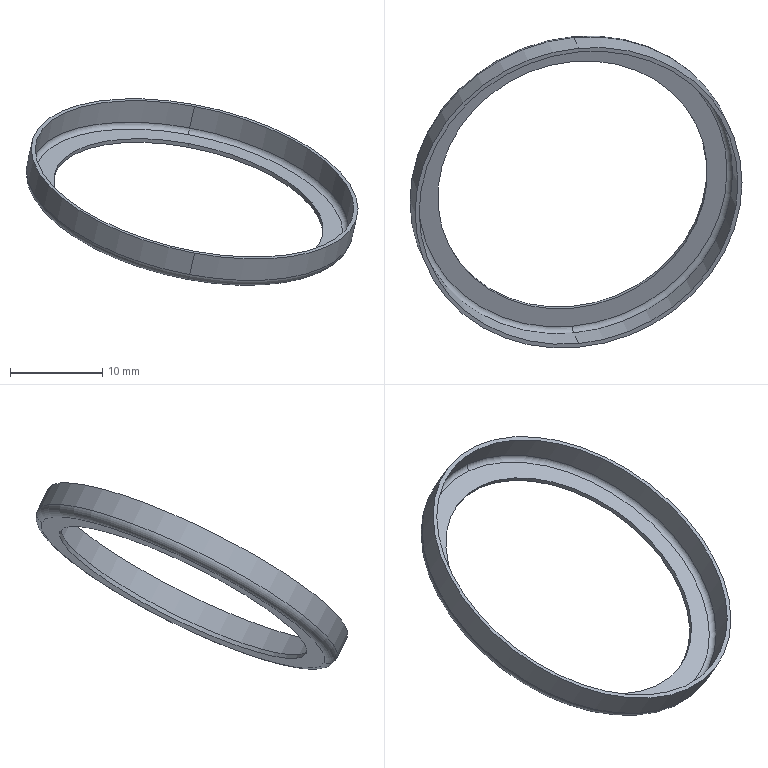Part | SolidWorks | features BaseBody 1 | 1 solid | 13 faces | box 35.944 x 33.77 x 20.198 mm | volume 291.989 mm3 | cylinder 6 | torus 4 | plane 3 | commonest cylinder face diameters 29.8 x2 35.23 x2 36.13 x2
STEP:
#1=CARTESIAN_POINT('',(1945.708,-185.265,909.185));
#2=VERTEX_POINT('',#1);
#3=CARTESIAN_POINT('',(1945.708,-211.95,895.919));
#4=VERTEX_POINT('',#3);
#5=CARTESIAN_POINT('',(1945.708,-198.607,902.552));
#6=DIRECTION('',(0.2015,-0.436,0.8771));
#7=DIRECTION('',(0.,-0.8955,-0.4451));
#8=AXIS2_PLACEMENT_3D('',#5,#6,#7);
#9=CIRCLE('',#8,14.9);
#10=EDGE_CURVE('',#2,#4,#9,.T.);
#11=ORIENTED_EDGE('',*,*,#10,.F.);
#12=CARTESIAN_POINT('',(1945.799,-185.461,909.579));
#13=VERTEX_POINT('',#12);
#14=CARTESIAN_POINT('',(1943.539,-180.572,899.743));
#15=DIRECTION('',(0.2015,-0.436,0.8771));
#16=VECTOR('',#15,1000.);
#17=LINE('',#14,#16);
#18=EDGE_CURVE('',#2,#13,#17,.T.);
#19=ORIENTED_EDGE('',*,*,#18,.T.);
#20=CARTESIAN_POINT('',(1945.799,-212.146,896.314));
#21=VERTEX_POINT('',#20);
#22=CARTESIAN_POINT('',(1945.799,-198.804,902.947));
#23=DIRECTION('',(0.2015,-0.436,0.8771));
#24=DIRECTION('',(0.,-0.8955,-0.4451));
#25=AXIS2_PLACEMENT_3D('',#22,#23,#24);
#26=CIRCLE('',#25,14.9);
#27=EDGE_CURVE('',#13,#21,#26,.T.);
#28=ORIENTED_EDGE('',*,*,#27,.T.);
#29=CARTESIAN_POINT('',(1943.539,-207.256,886.478));
#30=DIRECTION('',(0.2015,-0.436,0.8771));
#31=VECTOR('',#30,1000.);
#32=LINE('',#29,#31);
#33=EDGE_CURVE('',#4,#21,#32,.T.);
#34=ORIENTED_EDGE('',*,*,#33,.F.);
#35=EDGE_LOOP('',(#11,#19,#28,#34));
#36=FACE_OUTER_BOUND('',#35,.T.);
#37=CARTESIAN_POINT('',(1943.539,-193.914,893.11));
#38=DIRECTION('',(0.2015,-0.436,0.8771));
#39=DIRECTION('',(0.,-0.8955,-0.4451));
#40=AXIS2_PLACEMENT_3D('',#37,#38,#39);
#41=CYLINDRICAL_SURFACE('',#40,14.9);
#42=ADVANCED_FACE('',(#36),#41,.F.);
#43=CARTESIAN_POINT('',(1945.799,-183.523,910.543));
#44=VERTEX_POINT('',#43);
#45=CARTESIAN_POINT('',(1945.799,-214.085,895.35));
#46=VERTEX_POINT('',#45);
#47=CARTESIAN_POINT('',(1945.799,-198.804,902.947));
#48=DIRECTION('',(0.2015,-0.436,0.8771));
#49=DIRECTION('',(0.,-0.8955,-0.4451));
#50=AXIS2_PLACEMENT_3D('',#47,#48,#49);
#51=CIRCLE('',#50,17.065);
#52=EDGE_CURVE('',#44,#46,#51,.T.);
#53=ORIENTED_EDGE('',*,*,#52,.F.);
#54=CARTESIAN_POINT('',(1945.909,-183.27,911.27));
#55=VERTEX_POINT('',#54);
#56=CARTESIAN_POINT('',(1945.909,-183.762,911.025));
#57=DIRECTION('',(0.9795,0.08968,-0.1804));
#58=DIRECTION('',(-0.1811,0.,-0.9835));
#59=AXIS2_PLACEMENT_3D('',#56,#57,#58);
#60=CIRCLE('',#59,0.55);
#61=EDGE_CURVE('',#44,#55,#60,.T.);
#62=ORIENTED_EDGE('',*,*,#61,.T.);
#63=CARTESIAN_POINT('',(1945.909,-214.817,895.588));
#64=VERTEX_POINT('',#63);
#65=CARTESIAN_POINT('',(1945.909,-199.043,903.429));
#66=DIRECTION('',(0.2015,-0.436,0.8771));
#67=DIRECTION('',(0.,-0.8955,-0.4451));
#68=AXIS2_PLACEMENT_3D('',#65,#66,#67);
#69=CIRCLE('',#68,17.615);
#70=EDGE_CURVE('',#55,#64,#69,.T.);
#71=ORIENTED_EDGE('',*,*,#70,.T.);
#72=CARTESIAN_POINT('',(1945.909,-214.324,895.833));
#73=DIRECTION('',(-0.9795,-0.08968,0.1804));
#74=DIRECTION('',(0.1811,0.,0.9835));
#75=AXIS2_PLACEMENT_3D('',#72,#73,#74);
#76=CIRCLE('',#75,0.55);
#77=EDGE_CURVE('',#46,#64,#76,.T.);
#78=ORIENTED_EDGE('',*,*,#77,.F.);
#79=EDGE_LOOP('',(#53,#62,#71,#78));
#80=FACE_OUTER_BOUND('',#79,.T.);
#81=CARTESIAN_POINT('',(1945.909,-199.043,903.429));
#82=DIRECTION('',(0.2015,-0.436,0.8771));
#83=DIRECTION('',(0.,-0.8955,-0.4451));
#84=AXIS2_PLACEMENT_3D('',#81,#82,#83);
#85=TOROIDAL_SURFACE('',#84,17.065,0.55);
#86=ADVANCED_FACE('',(#80),#85,.F.);
#87=ORIENTED_EDGE('',*,*,#70,.F.);
#88=CARTESIAN_POINT('',(1946.443,-184.425,913.595));
#89=VERTEX_POINT('',#88);
#90=CARTESIAN_POINT('',(1943.539,-178.14,900.951));
#91=DIRECTION('',(0.2015,-0.436,0.8771));
#92=VECTOR('',#91,1000.);
#93=LINE('',#90,#92);
#94=EDGE_CURVE('',#55,#89,#93,.T.);
#95=ORIENTED_EDGE('',*,*,#94,.T.);
#96=CARTESIAN_POINT('',(1946.443,-215.972,897.912));
#97=VERTEX_POINT('',#96);
#98=CARTESIAN_POINT('',(1946.443,-200.199,905.753));
#99=DIRECTION('',(0.2015,-0.436,0.8771));
#100=DIRECTION('',(0.,-0.8955,-0.4451));
#101=AXIS2_PLACEMENT_3D('',#98,#99,#100);
#102=CIRCLE('',#101,17.615);
#103=EDGE_CURVE('',#89,#97,#102,.T.);
#104=ORIENTED_EDGE('',*,*,#103,.T.);
#105=CARTESIAN_POINT('',(1943.539,-209.687,885.269));
#106=DIRECTION('',(0.2015,-0.436,0.8771));
#107=VECTOR('',#106,1000.);
#108=LINE('',#105,#107);
#109=EDGE_CURVE('',#64,#97,#108,.T.);
#110=ORIENTED_EDGE('',*,*,#109,.F.);
#111=EDGE_LOOP('',(#87,#95,#104,#110));
#112=FACE_OUTER_BOUND('',#111,.T.);
#113=CARTESIAN_POINT('',(1943.539,-193.914,893.11));
#114=DIRECTION('',(0.2015,-0.436,0.8771));
#115=DIRECTION('',(0.,-0.8955,-0.4451));
#116=AXIS2_PLACEMENT_3D('',#113,#114,#115);
#117=CYLINDRICAL_SURFACE('',#116,17.615);
#118=ADVANCED_FACE('',(#112),#117,.F.);
#119=CARTESIAN_POINT('',(1945.909,-215.22,895.387));
#120=VERTEX_POINT('',#119);
#121=CARTESIAN_POINT('',(1945.909,-182.867,911.471));
#122=VERTEX_POINT('',#121);
#123=CARTESIAN_POINT('',(1945.909,-199.043,903.429));
#124=DIRECTION('',(0.2015,-0.436,0.8771));
#125=DIRECTION('',(0.,-0.8955,-0.4451));
#126=AXIS2_PLACEMENT_3D('',#123,#124,#125);
#127=CIRCLE('',#126,18.065);
#128=EDGE_CURVE('',#120,#122,#127,.T.);
#129=ORIENTED_EDGE('',*,*,#128,.T.);
#130=CARTESIAN_POINT('',(1946.443,-184.022,913.795));
#131=VERTEX_POINT('',#130);
#132=CARTESIAN_POINT('',(1943.539,-177.737,901.152));
#133=DIRECTION('',(0.2015,-0.436,0.8771));
#134=VECTOR('',#133,1000.);
#135=LINE('',#132,#134);
#136=EDGE_CURVE('',#122,#131,#135,.T.);
#137=ORIENTED_EDGE('',*,*,#136,.T.);
#138=CARTESIAN_POINT('',(1946.443,-216.375,897.712));
#139=VERTEX_POINT('',#138);
#140=CARTESIAN_POINT('',(1946.443,-200.199,905.753));
#141=DIRECTION('',(0.2015,-0.436,0.8771));
#142=DIRECTION('',(0.,-0.8955,-0.4451));
#143=AXIS2_PLACEMENT_3D('',#140,#141,#142);
#144=CIRCLE('',#143,18.065);
#145=EDGE_CURVE('',#139,#131,#144,.T.);
#146=ORIENTED_EDGE('',*,*,#145,.F.);
#147=CARTESIAN_POINT('',(1943.539,-210.09,885.069));
#148=DIRECTION('',(0.2015,-0.436,0.8771));
#149=VECTOR('',#148,1000.);
#150=LINE('',#147,#149);
#151=EDGE_CURVE('',#120,#139,#150,.T.);
#152=ORIENTED_EDGE('',*,*,#151,.F.);
#153=EDGE_LOOP('',(#129,#137,#146,#152));
#154=FACE_OUTER_BOUND('',#153,.T.);
#155=CARTESIAN_POINT('',(1943.539,-193.914,893.11));
#156=DIRECTION('',(0.2015,-0.436,0.8771));
#157=DIRECTION('',(0.,-0.8955,-0.4451));
#158=AXIS2_PLACEMENT_3D('',#155,#156,#157);
#159=CYLINDRICAL_SURFACE('',#158,18.065);
#160=ADVANCED_FACE('',(#154),#159,.T.);
#161=CARTESIAN_POINT('',(1945.708,-213.888,894.956));
#162=VERTEX_POINT('',#161);
#163=CARTESIAN_POINT('',(1945.708,-183.326,910.148));
#164=VERTEX_POINT('',#163);
#165=CARTESIAN_POINT('',(1945.708,-198.607,902.552));
#166=DIRECTION('',(0.2015,-0.436,0.8771));
#167=DIRECTION('',(0.,-0.8955,-0.4451));
#168=AXIS2_PLACEMENT_3D('',#165,#166,#167);
#169=CIRCLE('',#168,17.065);
#170=EDGE_CURVE('',#162,#164,#169,.T.);
#171=ORIENTED_EDGE('',*,*,#170,.T.);
#172=CARTESIAN_POINT('',(1945.909,-183.762,911.025));
#173=DIRECTION('',(0.9795,0.08968,-0.1804));
#174=DIRECTION('',(-0.1811,0.,-0.9835));
#175=AXIS2_PLACEMENT_3D('',#172,#173,#174);
#176=CIRCLE('',#175,1.);
#177=EDGE_CURVE('',#164,#122,#176,.T.);
#178=ORIENTED_EDGE('',*,*,#177,.T.);
#179=ORIENTED_EDGE('',*,*,#128,.F.);
#180=CARTESIAN_POINT('',(1945.909,-214.324,895.833));
#181=DIRECTION('',(-0.9795,-0.08968,0.1804));
#182=DIRECTION('',(0.1811,0.,0.9835));
#183=AXIS2_PLACEMENT_3D('',#180,#181,#182);
#184=CIRCLE('',#183,1.);
#185=EDGE_CURVE('',#162,#120,#184,.T.);
#186=ORIENTED_EDGE('',*,*,#185,.F.);
#187=EDGE_LOOP('',(#171,#178,#179,#186));
#188=FACE_OUTER_BOUND('',#187,.T.);
#189=CARTESIAN_POINT('',(1945.909,-199.043,903.429));
#190=DIRECTION('',(0.2015,-0.436,0.8771));
#191=DIRECTION('',(0.,-0.8955,-0.4451));
#192=AXIS2_PLACEMENT_3D('',#189,#190,#191);
#193=TOROIDAL_SURFACE('',#192,17.065,1.);
#194=ADVANCED_FACE('',(#188),#193,.T.);
#195=ORIENTED_EDGE('',*,*,#177,.F.);
#196=CARTESIAN_POINT('',(1945.708,-198.607,902.552));
#197=DIRECTION('',(0.2015,-0.436,0.8771));
#198=DIRECTION('',(0.,-0.8955,-0.4451));
#199=AXIS2_PLACEMENT_3D('',#196,#197,#198);
#200=CIRCLE('',#199,17.065);
#201=EDGE_CURVE('',#164,#162,#200,.T.);
#202=ORIENTED_EDGE('',*,*,#201,.T.);
#203=ORIENTED_EDGE('',*,*,#185,.T.);
#204=CARTESIAN_POINT('',(1945.909,-199.043,903.429));
#205=DIRECTION('',(0.2015,-0.436,0.8771));
#206=DIRECTION('',(0.,-0.8955,-0.4451));
#207=AXIS2_PLACEMENT_3D('',#204,#205,#206);
#208=CIRCLE('',#207,18.065);
#209=EDGE_CURVE('',#122,#120,#208,.T.);
#210=ORIENTED_EDGE('',*,*,#209,.F.);
#211=EDGE_LOOP('',(#195,#202,#203,#210));
#212=FACE_OUTER_BOUND('',#211,.T.);
#213=CARTESIAN_POINT('',(1945.909,-199.043,903.429));
#214=DIRECTION('',(0.2015,-0.436,0.8771));
#215=DIRECTION('',(0.,-0.8955,-0.4451));
#216=AXIS2_PLACEMENT_3D('',#213,#214,#215);
#217=TOROIDAL_SURFACE('',#216,17.065,1.);
#218=ADVANCED_FACE('',(#212),#217,.T.);
#219=ORIENTED_EDGE('',*,*,#136,.F.);
#220=ORIENTED_EDGE('',*,*,#209,.T.);
#221=ORIENTED_EDGE('',*,*,#151,.T.);
#222=CARTESIAN_POINT('',(1946.443,-200.199,905.753));
#223=DIRECTION('',(0.2015,-0.436,0.8771));
#224=DIRECTION('',(0.,-0.8955,-0.4451));
#225=AXIS2_PLACEMENT_3D('',#222,#223,#224);
#226=CIRCLE('',#225,18.065);
#227=EDGE_CURVE('',#131,#139,#226,.T.);
#228=ORIENTED_EDGE('',*,*,#227,.F.);
#229=EDGE_LOOP('',(#219,#220,#221,#228));
#230=FACE_OUTER_BOUND('',#229,.T.);
#231=CARTESIAN_POINT('',(1943.539,-193.914,893.11));
#232=DIRECTION('',(0.2015,-0.436,0.8771));
#233=DIRECTION('',(0.,-0.8955,-0.4451));
#234=AXIS2_PLACEMENT_3D('',#231,#232,#233);
#235=CYLINDRICAL_SURFACE('',#234,18.065);
#236=ADVANCED_FACE('',(#230),#235,.T.);
#237=CARTESIAN_POINT('',(1946.443,-200.199,905.753));
#238=DIRECTION('',(0.2015,-0.436,0.8771));
#239=DIRECTION('',(0.,-0.8955,-0.4451));
#240=AXIS2_PLACEMENT_3D('',#237,#238,#239);
#241=CIRCLE('',#240,17.615);
#242=EDGE_CURVE('',#97,#89,#241,.T.);
#243=ORIENTED_EDGE('',*,*,#242,.F.);
#244=ORIENTED_EDGE('',*,*,#103,.F.);
#245=EDGE_LOOP('',(#243,#244));
#246=FACE_BOUND('',#245,.T.);
#247=ORIENTED_EDGE('',*,*,#145,.T.);
#248=ORIENTED_EDGE('',*,*,#227,.T.);
#249=EDGE_LOOP('',(#247,#248));
#250=FACE_OUTER_BOUND('',#249,.T.);
#251=CARTESIAN_POINT('',(1931.838,-192.405,912.983));
#252=DIRECTION('',(-0.2015,0.436,-0.8771));
#253=DIRECTION('',(0.,0.8955,0.4451));
#254=AXIS2_PLACEMENT_3D('',#251,#252,#253);
#255=PLANE('',#254);
#256=ADVANCED_FACE('',(#246,#250),#255,.F.);
#257=ORIENTED_EDGE('',*,*,#94,.F.);
#258=CARTESIAN_POINT('',(1945.909,-199.043,903.429));
#259=DIRECTION('',(0.2015,-0.436,0.8771));
#260=DIRECTION('',(0.,-0.8955,-0.4451));
#261=AXIS2_PLACEMENT_3D('',#258,#259,#260);
#262=CIRCLE('',#261,17.615);
#263=EDGE_CURVE('',#64,#55,#262,.T.);
#264=ORIENTED_EDGE('',*,*,#263,.F.);
#265=ORIENTED_EDGE('',*,*,#109,.T.);
#266=ORIENTED_EDGE('',*,*,#242,.T.);
#267=EDGE_LOOP('',(#257,#264,#265,#266));
#268=FACE_OUTER_BOUND('',#267,.T.);
#269=CARTESIAN_POINT('',(1943.539,-193.914,893.11));
#270=DIRECTION('',(0.2015,-0.436,0.8771));
#271=DIRECTION('',(0.,-0.8955,-0.4451));
#272=AXIS2_PLACEMENT_3D('',#269,#270,#271);
#273=CYLINDRICAL_SURFACE('',#272,17.615);
#274=ADVANCED_FACE('',(#268),#273,.F.);
#275=ORIENTED_EDGE('',*,*,#61,.F.);
#276=CARTESIAN_POINT('',(1945.799,-198.804,902.947));
#277=DIRECTION('',(0.2015,-0.436,0.8771));
#278=DIRECTION('',(0.,-0.8955,-0.4451));
#279=AXIS2_PLACEMENT_3D('',#276,#277,#278);
#280=CIRCLE('',#279,17.065);
#281=EDGE_CURVE('',#46,#44,#280,.T.);
#282=ORIENTED_EDGE('',*,*,#281,.F.);
#283=ORIENTED_EDGE('',*,*,#77,.T.);
#284=ORIENTED_EDGE('',*,*,#263,.T.);
#285=EDGE_LOOP('',(#275,#282,#283,#284));
#286=FACE_OUTER_BOUND('',#285,.T.);
#287=CARTESIAN_POINT('',(1945.909,-199.043,903.429));
#288=DIRECTION('',(0.2015,-0.436,0.8771));
#289=DIRECTION('',(0.,-0.8955,-0.4451));
#290=AXIS2_PLACEMENT_3D('',#287,#288,#289);
#291=TOROIDAL_SURFACE('',#290,17.065,0.55);
#292=ADVANCED_FACE('',(#286),#291,.F.);
#293=CARTESIAN_POINT('',(1945.799,-198.804,902.947));
#294=DIRECTION('',(0.2015,-0.436,0.8771));
#295=DIRECTION('',(0.,-0.8955,-0.4451));
#296=AXIS2_PLACEMENT_3D('',#293,#294,#295);
#297=CIRCLE('',#296,14.9);
#298=EDGE_CURVE('',#21,#13,#297,.T.);
#299=ORIENTED_EDGE('',*,*,#298,.F.);
#300=ORIENTED_EDGE('',*,*,#27,.F.);
#301=EDGE_LOOP('',(#299,#300));
#302=FACE_BOUND('',#301,.T.);
#303=ORIENTED_EDGE('',*,*,#281,.T.);
#304=ORIENTED_EDGE('',*,*,#52,.T.);
#305=EDGE_LOOP('',(#303,#304));
#306=FACE_OUTER_BOUND('',#305,.T.);
#307=CARTESIAN_POINT('',(1932.001,-191.441,909.776));
#308=DIRECTION('',(-0.2015,0.436,-0.8771));
#309=DIRECTION('',(0.,0.8955,0.4451));
#310=AXIS2_PLACEMENT_3D('',#307,#308,#309);
#311=PLANE('',#310);
#312=ADVANCED_FACE('',(#302,#306),#311,.F.);
#313=ORIENTED_EDGE('',*,*,#18,.F.);
#314=CARTESIAN_POINT('',(1945.708,-198.607,902.552));
#315=DIRECTION('',(0.2015,-0.436,0.8771));
#316=DIRECTION('',(0.,-0.8955,-0.4451));
#317=AXIS2_PLACEMENT_3D('',#314,#315,#316);
#318=CIRCLE('',#317,14.9);
#319=EDGE_CURVE('',#4,#2,#318,.T.);
#320=ORIENTED_EDGE('',*,*,#319,.F.);
#321=ORIENTED_EDGE('',*,*,#33,.T.);
#322=ORIENTED_EDGE('',*,*,#298,.T.);
#323=EDGE_LOOP('',(#313,#320,#321,#322));
#324=FACE_OUTER_BOUND('',#323,.T.);
#325=CARTESIAN_POINT('',(1943.539,-193.914,893.11));
#326=DIRECTION('',(0.2015,-0.436,0.8771));
#327=DIRECTION('',(0.,-0.8955,-0.4451));
#328=AXIS2_PLACEMENT_3D('',#325,#326,#327);
#329=CYLINDRICAL_SURFACE('',#328,14.9);
#330=ADVANCED_FACE('',(#324),#329,.F.);
#331=ORIENTED_EDGE('',*,*,#170,.F.);
#332=ORIENTED_EDGE('',*,*,#201,.F.);
#333=EDGE_LOOP('',(#331,#332));
#334=FACE_OUTER_BOUND('',#333,.T.);
#335=ORIENTED_EDGE('',*,*,#319,.T.);
#336=ORIENTED_EDGE('',*,*,#10,.T.);
#337=EDGE_LOOP('',(#335,#336));
#338=FACE_BOUND('',#337,.T.);
#339=CARTESIAN_POINT('',(1933.661,-192.179,908.515));
#340=DIRECTION('',(0.2015,-0.436,0.8771));
#341=DIRECTION('',(0.,-0.8955,-0.4451));
#342=AXIS2_PLACEMENT_3D('',#339,#340,#341);
#343=PLANE('',#342);
#344=ADVANCED_FACE('',(#334,#338),#343,.F.);
#345=CLOSED_SHELL('',(#42,#86,#118,#160,#194,#218,#236,#256,#274,#292,#312,#330,#344));
#346=MANIFOLD_SOLID_BREP('',#345);
#347=CARTESIAN_POINT('',(0.,0.,0.));
#348=DIRECTION('',(0.,0.,1.));
#349=DIRECTION('',(1.,0.,0.));
#350=AXIS2_PLACEMENT_3D('',#347,#348,#349);
#351=(LENGTH_UNIT()NAMED_UNIT(*)SI_UNIT(.MILLI.,.METRE.));
#352=UNCERTAINTY_MEASURE_WITH_UNIT(LENGTH_MEASURE(0.00001),#351,'','');
#353=(NAMED_UNIT(*)PLANE_ANGLE_UNIT()SI_UNIT($,.RADIAN.));
#354=(NAMED_UNIT(*)SI_UNIT($,.STERADIAN.)SOLID_ANGLE_UNIT());
#355=(GEOMETRIC_REPRESENTATION_CONTEXT(3)GLOBAL_UNCERTAINTY_ASSIGNED_CONTEXT((#352))GLOBAL_UNIT_ASSIGNED_CONTEXT((#351,#353,#354))REPRESENTATION_CONTEXT('',''));
#356=ADVANCED_BREP_SHAPE_REPRESENTATION('',(#346,#350),#355);